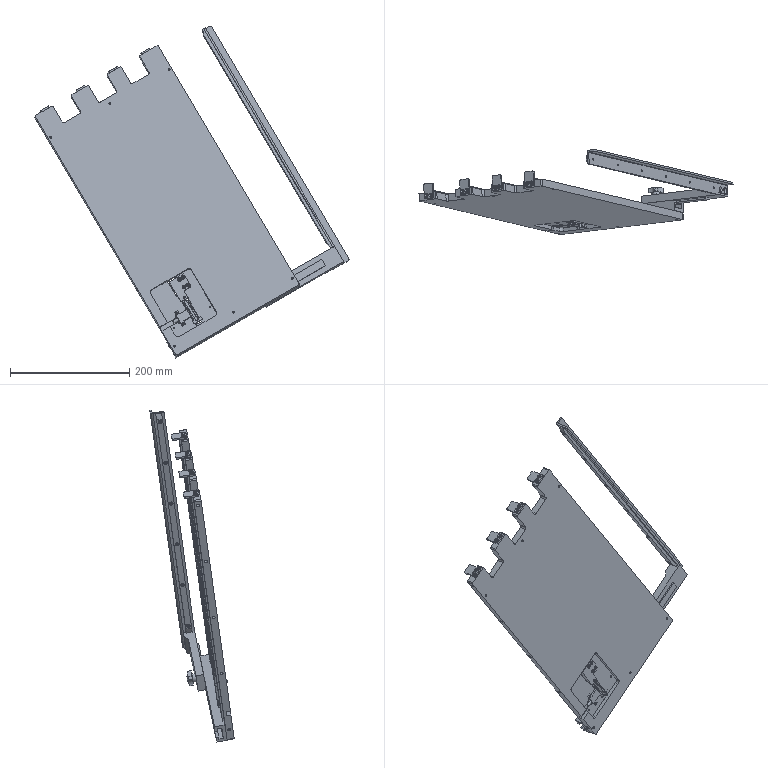Part | NX | features BREP 15 | 20 solids | 763 faces | box 527.078 x 141.718 x 557.213 mm | volume 1563521 mm3 | cylinder 332 | plane 243 | cone 183 | spline 4 | sphere 1 | commonest cylinder face diameters 2.5 x94 3.4 x84 4 x41 5 x20 3 x18 4.5 x17